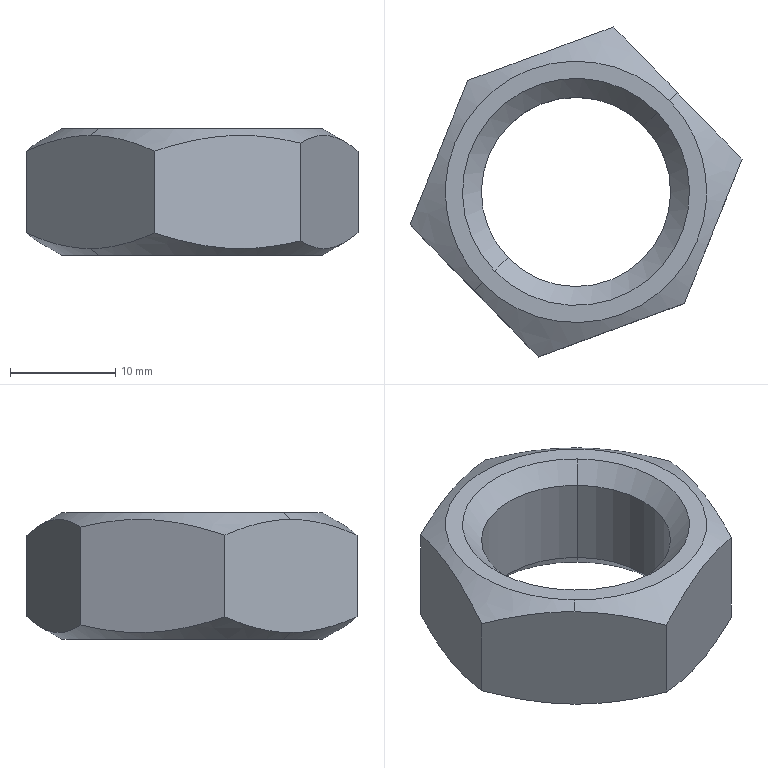Part | SolidWorks | features BaseBody 1 | 1 solid | 18 faces | box 31.577 x 31.388 x 12 mm | volume 4193 mm3 | cone 8 | plane 8 | cylinder 2 | commonest cylinder face diameters 18 x2
STEP:
#1=CARTESIAN_POINT('',(-38.01,-43.83,139.05));
#2=VERTEX_POINT('',#1);
#3=CARTESIAN_POINT('',(-50.916,-56.377,139.05));
#4=VERTEX_POINT('',#3);
#5=CARTESIAN_POINT('',(-44.463,-50.104,139.05));
#6=DIRECTION('',(0.,0.,1.));
#7=DIRECTION('',(-0.717,-0.697,0.));
#8=AXIS2_PLACEMENT_3D('',#5,#6,#7);
#9=CIRCLE('',#8,9.);
#10=EDGE_CURVE('',#2,#4,#9,.T.);
#11=ORIENTED_EDGE('',*,*,#10,.T.);
#12=CARTESIAN_POINT('',(-50.916,-56.377,130.65));
#13=VERTEX_POINT('',#12);
#14=CARTESIAN_POINT('',(-50.916,-56.377,140.85));
#15=DIRECTION('',(0.,0.,-1.));
#16=VECTOR('',#15,1000.);
#17=LINE('',#14,#16);
#18=EDGE_CURVE('',#4,#13,#17,.T.);
#19=ORIENTED_EDGE('',*,*,#18,.T.);
#20=CARTESIAN_POINT('',(-38.01,-43.83,130.65));
#21=VERTEX_POINT('',#20);
#22=CARTESIAN_POINT('',(-44.463,-50.104,130.65));
#23=DIRECTION('',(0.,0.,-1.));
#24=DIRECTION('',(-0.717,-0.697,0.));
#25=AXIS2_PLACEMENT_3D('',#22,#23,#24);
#26=CIRCLE('',#25,9.);
#27=EDGE_CURVE('',#13,#21,#26,.T.);
#28=ORIENTED_EDGE('',*,*,#27,.T.);
#29=CARTESIAN_POINT('',(-38.01,-43.83,140.85));
#30=DIRECTION('',(0.,0.,-1.));
#31=VECTOR('',#30,1000.);
#32=LINE('',#29,#31);
#33=EDGE_CURVE('',#2,#21,#32,.T.);
#34=ORIENTED_EDGE('',*,*,#33,.F.);
#35=EDGE_LOOP('',(#11,#19,#28,#34));
#36=FACE_OUTER_BOUND('',#35,.T.);
#37=CARTESIAN_POINT('',(-44.463,-50.104,140.85));
#38=DIRECTION('',(0.,0.,-1.));
#39=DIRECTION('',(0.717,0.697,0.));
#40=AXIS2_PLACEMENT_3D('',#37,#38,#39);
#41=CYLINDRICAL_SURFACE('',#40,9.);
#42=ADVANCED_FACE('',(#36),#41,.F.);
#43=ORIENTED_EDGE('',*,*,#10,.F.);
#44=CARTESIAN_POINT('',(-36.719,-42.576,140.85));
#45=VERTEX_POINT('',#44);
#46=CARTESIAN_POINT('',(-38.01,-43.83,139.05));
#47=DIRECTION('',(0.507,0.4929,0.7071));
#48=VECTOR('',#47,1000.);
#49=LINE('',#46,#48);
#50=EDGE_CURVE('',#2,#45,#49,.T.);
#51=ORIENTED_EDGE('',*,*,#50,.T.);
#52=CARTESIAN_POINT('',(-52.207,-57.632,140.85));
#53=VERTEX_POINT('',#52);
#54=CARTESIAN_POINT('',(-44.463,-50.104,140.85));
#55=DIRECTION('',(0.,0.,-1.));
#56=DIRECTION('',(-0.717,-0.697,0.));
#57=AXIS2_PLACEMENT_3D('',#54,#55,#56);
#58=CIRCLE('',#57,10.8);
#59=EDGE_CURVE('',#53,#45,#58,.T.);
#60=ORIENTED_EDGE('',*,*,#59,.F.);
#61=CARTESIAN_POINT('',(-50.916,-56.377,139.05));
#62=DIRECTION('',(-0.507,-0.4929,0.7071));
#63=VECTOR('',#62,1000.);
#64=LINE('',#61,#63);
#65=EDGE_CURVE('',#4,#53,#64,.T.);
#66=ORIENTED_EDGE('',*,*,#65,.F.);
#67=EDGE_LOOP('',(#43,#51,#60,#66));
#68=FACE_OUTER_BOUND('',#67,.T.);
#69=CARTESIAN_POINT('',(-44.463,-50.104,139.05));
#70=DIRECTION('',(0.,0.,1.));
#71=DIRECTION('',(-0.717,-0.697,0.));
#72=AXIS2_PLACEMENT_3D('',#69,#70,#71);
#73=CONICAL_SURFACE('',#72,9.,0.7854);
#74=ADVANCED_FACE('',(#68),#73,.F.);
#75=ORIENTED_EDGE('',*,*,#27,.F.);
#76=CARTESIAN_POINT('',(-52.207,-57.632,128.85));
#77=VERTEX_POINT('',#76);
#78=CARTESIAN_POINT('',(-52.207,-57.632,128.85));
#79=DIRECTION('',(-0.507,-0.4929,-0.7071));
#80=VECTOR('',#79,1000.);
#81=LINE('',#78,#80);
#82=EDGE_CURVE('',#13,#77,#81,.T.);
#83=ORIENTED_EDGE('',*,*,#82,.T.);
#84=CARTESIAN_POINT('',(-36.719,-42.576,128.85));
#85=VERTEX_POINT('',#84);
#86=CARTESIAN_POINT('',(-44.463,-50.104,128.85));
#87=DIRECTION('',(0.,0.,1.));
#88=DIRECTION('',(-0.717,-0.697,0.));
#89=AXIS2_PLACEMENT_3D('',#86,#87,#88);
#90=CIRCLE('',#89,10.8);
#91=EDGE_CURVE('',#85,#77,#90,.T.);
#92=ORIENTED_EDGE('',*,*,#91,.F.);
#93=CARTESIAN_POINT('',(-36.719,-42.576,128.85));
#94=DIRECTION('',(0.507,0.4929,-0.7071));
#95=VECTOR('',#94,1000.);
#96=LINE('',#93,#95);
#97=EDGE_CURVE('',#21,#85,#96,.T.);
#98=ORIENTED_EDGE('',*,*,#97,.F.);
#99=EDGE_LOOP('',(#75,#83,#92,#98));
#100=FACE_OUTER_BOUND('',#99,.T.);
#101=CARTESIAN_POINT('',(-44.463,-50.104,128.85));
#102=DIRECTION('',(0.,0.,-1.));
#103=DIRECTION('',(0.717,0.697,0.));
#104=AXIS2_PLACEMENT_3D('',#101,#102,#103);
#105=CONICAL_SURFACE('',#104,10.8,0.7854);
#106=ADVANCED_FACE('',(#100),#105,.F.);
#107=CARTESIAN_POINT('',(-53.372,-58.765,128.85));
#108=VERTEX_POINT('',#107);
#109=CARTESIAN_POINT('',(-35.554,-41.443,128.85));
#110=VERTEX_POINT('',#109);
#111=CARTESIAN_POINT('',(-44.463,-50.104,128.85));
#112=DIRECTION('',(0.,0.,-1.));
#113=DIRECTION('',(0.717,0.697,0.));
#114=AXIS2_PLACEMENT_3D('',#111,#112,#113);
#115=CIRCLE('',#114,12.425);
#116=EDGE_CURVE('',#108,#110,#115,.T.);
#117=ORIENTED_EDGE('',*,*,#116,.F.);
#118=CARTESIAN_POINT('',(-54.143,-59.514,129.471));
#119=VERTEX_POINT('',#118);
#120=CARTESIAN_POINT('',(-53.372,-58.765,128.85));
#121=DIRECTION('',(-0.621,-0.6037,0.5));
#122=VECTOR('',#121,1000.);
#123=LINE('',#120,#122);
#124=EDGE_CURVE('',#108,#119,#123,.T.);
#125=ORIENTED_EDGE('',*,*,#124,.T.);
#126=CARTESIAN_POINT('',(-60.251,-53.23,130.969));
#127=VERTEX_POINT('',#126);
#128=CARTESIAN_POINT('',(-54.143,-59.514,129.471));
#129=CARTESIAN_POINT('',(-55.19,-58.437,129.471));
#130=CARTESIAN_POINT('',(-56.22,-57.377,129.618));
#131=CARTESIAN_POINT('',(-58.253,-55.286,130.144));
#132=CARTESIAN_POINT('',(-59.256,-54.254,130.52));
#133=CARTESIAN_POINT('',(-60.251,-53.23,130.969));
#134=B_SPLINE_CURVE_WITH_KNOTS('',3,(#128,#129,#130,#131,#132,#133),.UNSPECIFIED.,.F.,.F.,(4,2,4),(0.008891,0.01334,0.0178),.UNSPECIFIED.);
#135=EDGE_CURVE('',#119,#127,#134,.T.);
#136=ORIENTED_EDGE('',*,*,#135,.T.);
#137=CARTESIAN_POINT('',(-54.765,-39.506,130.21));
#138=VERTEX_POINT('',#137);
#139=CARTESIAN_POINT('',(-60.251,-53.23,130.969));
#140=CARTESIAN_POINT('',(-59.363,-51.008,130.217));
#141=CARTESIAN_POINT('',(-58.462,-48.754,129.669));
#142=CARTESIAN_POINT('',(-57.303,-45.855,129.477));
#143=CARTESIAN_POINT('',(-57.069,-45.269,129.463));
#144=CARTESIAN_POINT('',(-56.603,-44.103,129.487));
#145=CARTESIAN_POINT('',(-56.371,-43.522,129.524));
#146=CARTESIAN_POINT('',(-55.678,-41.789,129.706));
#147=CARTESIAN_POINT('',(-55.22,-40.643,129.922));
#148=CARTESIAN_POINT('',(-54.765,-39.506,130.21));
#149=B_SPLINE_CURVE_WITH_KNOTS('',3,(#139,#140,#141,#142,#143,#144,#145,#146,#147,#148),.UNSPECIFIED.,.F.,.F.,(4,2,2,2,4),(0.,0.007459,0.009324,0.01119,0.01492),.UNSPECIFIED.);
#150=EDGE_CURVE('',#127,#138,#149,.T.);
#151=ORIENTED_EDGE('',*,*,#150,.T.);
#152=CARTESIAN_POINT('',(-40.892,-34.41,130.969));
#153=VERTEX_POINT('',#152);
#154=CARTESIAN_POINT('',(-54.765,-39.506,130.21));
#155=CARTESIAN_POINT('',(-53.617,-39.084,129.922));
#156=CARTESIAN_POINT('',(-52.464,-38.661,129.707));
#157=CARTESIAN_POINT('',(-50.142,-37.808,129.464));
#158=CARTESIAN_POINT('',(-48.974,-37.379,129.438));
#159=CARTESIAN_POINT('',(-47.209,-36.731,129.55));
#160=CARTESIAN_POINT('',(-46.62,-36.514,129.613));
#161=CARTESIAN_POINT('',(-45.454,-36.086,129.782));
#162=CARTESIAN_POINT('',(-44.876,-35.874,129.889));
#163=CARTESIAN_POINT('',(-43.152,-35.24,130.266));
#164=CARTESIAN_POINT('',(-42.017,-34.823,130.592));
#165=CARTESIAN_POINT('',(-40.892,-34.41,130.969));
#166=B_SPLINE_CURVE_WITH_KNOTS('',3,(#154,#155,#156,#157,#158,#159,#160,#161,#162,#163,#164,#165),.UNSPECIFIED.,.F.,.F.,(4,2,2,2,2,4),(0.,0.003728,0.007455,0.009319,0.01118,0.01491),.UNSPECIFIED.);
#167=EDGE_CURVE('',#138,#153,#166,.T.);
#168=ORIENTED_EDGE('',*,*,#167,.T.);
#169=CARTESIAN_POINT('',(-34.783,-40.694,129.471));
#170=VERTEX_POINT('',#169);
#171=CARTESIAN_POINT('',(-40.892,-34.41,130.969));
#172=CARTESIAN_POINT('',(-39.898,-35.432,130.521));
#173=CARTESIAN_POINT('',(-38.895,-36.464,130.145));
#174=CARTESIAN_POINT('',(-37.37,-38.032,129.75));
#175=CARTESIAN_POINT('',(-36.858,-38.559,129.647));
#176=CARTESIAN_POINT('',(-35.827,-39.62,129.507));
#177=CARTESIAN_POINT('',(-35.306,-40.156,129.471));
#178=CARTESIAN_POINT('',(-34.783,-40.694,129.471));
#179=B_SPLINE_CURVE_WITH_KNOTS('',3,(#171,#172,#173,#174,#175,#176,#177,#178),.UNSPECIFIED.,.F.,.F.,(4,2,2,4),(0.,0.004445,0.006668,0.008891),.UNSPECIFIED.);
#180=EDGE_CURVE('',#153,#170,#179,.T.);
#181=ORIENTED_EDGE('',*,*,#180,.T.);
#182=CARTESIAN_POINT('',(-35.554,-41.443,128.85));
#183=DIRECTION('',(0.621,0.6037,0.5));
#184=VECTOR('',#183,1000.);
#185=LINE('',#182,#184);
#186=EDGE_CURVE('',#110,#170,#185,.T.);
#187=ORIENTED_EDGE('',*,*,#186,.F.);
#188=EDGE_LOOP('',(#117,#125,#136,#151,#168,#181,#187));
#189=FACE_OUTER_BOUND('',#188,.T.);
#190=CARTESIAN_POINT('',(-44.463,-50.104,128.85));
#191=DIRECTION('',(0.,0.,1.));
#192=DIRECTION('',(0.717,0.697,0.));
#193=AXIS2_PLACEMENT_3D('',#190,#191,#192);
#194=CONICAL_SURFACE('',#193,12.425,1.047);
#195=ADVANCED_FACE('',(#189),#194,.T.);
#196=CARTESIAN_POINT('',(-35.554,-41.443,140.85));
#197=VERTEX_POINT('',#196);
#198=CARTESIAN_POINT('',(-53.372,-58.765,140.85));
#199=VERTEX_POINT('',#198);
#200=CARTESIAN_POINT('',(-44.463,-50.104,140.85));
#201=DIRECTION('',(0.,0.,1.));
#202=DIRECTION('',(-0.717,-0.697,0.));
#203=AXIS2_PLACEMENT_3D('',#200,#201,#202);
#204=CIRCLE('',#203,12.425);
#205=EDGE_CURVE('',#197,#199,#204,.T.);
#206=ORIENTED_EDGE('',*,*,#205,.F.);
#207=CARTESIAN_POINT('',(-34.783,-40.694,140.229));
#208=VERTEX_POINT('',#207);
#209=CARTESIAN_POINT('',(-35.554,-41.443,140.85));
#210=DIRECTION('',(0.621,0.6037,-0.5));
#211=VECTOR('',#210,1000.);
#212=LINE('',#209,#211);
#213=EDGE_CURVE('',#197,#208,#212,.T.);
#214=ORIENTED_EDGE('',*,*,#213,.T.);
#215=CARTESIAN_POINT('',(-40.892,-34.41,138.731));
#216=VERTEX_POINT('',#215);
#217=CARTESIAN_POINT('',(-34.783,-40.694,140.229));
#218=CARTESIAN_POINT('',(-35.83,-39.616,140.229));
#219=CARTESIAN_POINT('',(-36.86,-38.557,140.082));
#220=CARTESIAN_POINT('',(-38.893,-36.466,139.556));
#221=CARTESIAN_POINT('',(-39.897,-35.433,139.18));
#222=CARTESIAN_POINT('',(-40.892,-34.41,138.731));
#223=B_SPLINE_CURVE_WITH_KNOTS('',3,(#217,#218,#219,#220,#221,#222),.UNSPECIFIED.,.F.,.F.,(4,2,4),(0.008891,0.01334,0.0178),.UNSPECIFIED.);
#224=EDGE_CURVE('',#208,#216,#223,.T.);
#225=ORIENTED_EDGE('',*,*,#224,.T.);
#226=CARTESIAN_POINT('',(-54.765,-39.506,139.49));
#227=VERTEX_POINT('',#226);
#228=CARTESIAN_POINT('',(-40.892,-34.41,138.731));
#229=CARTESIAN_POINT('',(-43.138,-35.235,139.483));
#230=CARTESIAN_POINT('',(-45.417,-36.072,140.031));
#231=CARTESIAN_POINT('',(-48.347,-37.149,140.223));
#232=CARTESIAN_POINT('',(-48.94,-37.366,140.237));
#233=CARTESIAN_POINT('',(-50.119,-37.799,140.213));
#234=CARTESIAN_POINT('',(-50.705,-38.015,140.176));
#235=CARTESIAN_POINT('',(-52.458,-38.659,139.994));
#236=CARTESIAN_POINT('',(-53.616,-39.084,139.778));
#237=CARTESIAN_POINT('',(-54.765,-39.506,139.49));
#238=B_SPLINE_CURVE_WITH_KNOTS('',3,(#228,#229,#230,#231,#232,#233,#234,#235,#236,#237),.UNSPECIFIED.,.F.,.F.,(4,2,2,2,4),(0.,0.007459,0.009324,0.01119,0.01492),.UNSPECIFIED.);
#239=EDGE_CURVE('',#216,#227,#238,.T.);
#240=ORIENTED_EDGE('',*,*,#239,.T.);
#241=CARTESIAN_POINT('',(-60.251,-53.23,138.731));
#242=VERTEX_POINT('',#241);
#243=CARTESIAN_POINT('',(-54.765,-39.506,139.49));
#244=CARTESIAN_POINT('',(-55.219,-40.642,139.778));
#245=CARTESIAN_POINT('',(-55.675,-41.783,139.993));
#246=CARTESIAN_POINT('',(-56.593,-44.08,140.236));
#247=CARTESIAN_POINT('',(-57.055,-45.235,140.262));
#248=CARTESIAN_POINT('',(-57.753,-46.98,140.15));
#249=CARTESIAN_POINT('',(-57.986,-47.563,140.087));
#250=CARTESIAN_POINT('',(-58.447,-48.716,139.918));
#251=CARTESIAN_POINT('',(-58.676,-49.289,139.811));
#252=CARTESIAN_POINT('',(-59.358,-50.995,139.434));
#253=CARTESIAN_POINT('',(-59.806,-52.117,139.108));
#254=CARTESIAN_POINT('',(-60.251,-53.23,138.731));
#255=B_SPLINE_CURVE_WITH_KNOTS('',3,(#243,#244,#245,#246,#247,#248,#249,#250,#251,#252,#253,#254),.UNSPECIFIED.,.F.,.F.,(4,2,2,2,2,4),(0.,0.003728,0.007455,0.009319,0.01118,0.01491),.UNSPECIFIED.);
#256=EDGE_CURVE('',#227,#242,#255,.T.);
#257=ORIENTED_EDGE('',*,*,#256,.T.);
#258=CARTESIAN_POINT('',(-54.143,-59.514,140.229));
#259=VERTEX_POINT('',#258);
#260=CARTESIAN_POINT('',(-60.251,-53.23,138.731));
#261=CARTESIAN_POINT('',(-59.257,-54.253,139.179));
#262=CARTESIAN_POINT('',(-58.255,-55.284,139.555));
#263=CARTESIAN_POINT('',(-56.73,-56.853,139.95));
#264=CARTESIAN_POINT('',(-56.218,-57.379,140.053));
#265=CARTESIAN_POINT('',(-55.187,-58.44,140.193));
#266=CARTESIAN_POINT('',(-54.666,-58.976,140.229));
#267=CARTESIAN_POINT('',(-54.143,-59.514,140.229));
#268=B_SPLINE_CURVE_WITH_KNOTS('',3,(#260,#261,#262,#263,#264,#265,#266,#267),.UNSPECIFIED.,.F.,.F.,(4,2,2,4),(0.,0.004445,0.006668,0.008891),.UNSPECIFIED.);
#269=EDGE_CURVE('',#242,#259,#268,.T.);
#270=ORIENTED_EDGE('',*,*,#269,.T.);
#271=CARTESIAN_POINT('',(-53.372,-58.765,140.85));
#272=DIRECTION('',(-0.621,-0.6037,-0.5));
#273=VECTOR('',#272,1000.);
#274=LINE('',#271,#273);
#275=EDGE_CURVE('',#199,#259,#274,.T.);
#276=ORIENTED_EDGE('',*,*,#275,.F.);
#277=EDGE_LOOP('',(#206,#214,#225,#240,#257,#270,#276));
#278=FACE_OUTER_BOUND('',#277,.T.);
#279=CARTESIAN_POINT('',(-44.463,-50.104,140.85));
#280=DIRECTION('',(0.,0.,-1.));
#281=DIRECTION('',(-0.717,-0.697,0.));
#282=AXIS2_PLACEMENT_3D('',#279,#280,#281);
#283=CONICAL_SURFACE('',#282,12.425,1.047);
#284=ADVANCED_FACE('',(#278),#283,.T.);
#285=ORIENTED_EDGE('',*,*,#213,.F.);
#286=CARTESIAN_POINT('',(-44.463,-50.104,140.85));
#287=DIRECTION('',(0.,0.,1.));
#288=DIRECTION('',(-0.717,-0.697,0.));
#289=AXIS2_PLACEMENT_3D('',#286,#287,#288);
#290=CIRCLE('',#289,12.425);
#291=EDGE_CURVE('',#199,#197,#290,.T.);
#292=ORIENTED_EDGE('',*,*,#291,.F.);
#293=ORIENTED_EDGE('',*,*,#275,.T.);
#294=CARTESIAN_POINT('',(-48.034,-65.798,138.731));
#295=VERTEX_POINT('',#294);
#296=CARTESIAN_POINT('',(-54.143,-59.514,140.229));
#297=CARTESIAN_POINT('',(-53.096,-60.591,140.229));
#298=CARTESIAN_POINT('',(-52.066,-61.651,140.082));
#299=CARTESIAN_POINT('',(-50.032,-63.742,139.556));
#300=CARTESIAN_POINT('',(-49.029,-64.774,139.18));
#301=CARTESIAN_POINT('',(-48.034,-65.798,138.731));
#302=B_SPLINE_CURVE_WITH_KNOTS('',3,(#296,#297,#298,#299,#300,#301),.UNSPECIFIED.,.F.,.F.,(4,2,4),(0.008891,0.01334,0.0178),.UNSPECIFIED.);
#303=EDGE_CURVE('',#259,#295,#302,.T.);
#304=ORIENTED_EDGE('',*,*,#303,.T.);
#305=CARTESIAN_POINT('',(-34.161,-60.701,139.49));
#306=VERTEX_POINT('',#305);
#307=CARTESIAN_POINT('',(-48.034,-65.798,138.731));
#308=CARTESIAN_POINT('',(-45.788,-64.973,139.483));
#309=CARTESIAN_POINT('',(-43.509,-64.135,140.031));
#310=CARTESIAN_POINT('',(-40.579,-63.059,140.223));
#311=CARTESIAN_POINT('',(-39.986,-62.841,140.237));
#312=CARTESIAN_POINT('',(-38.807,-62.408,140.213));
#313=CARTESIAN_POINT('',(-38.22,-62.193,140.176));
#314=CARTESIAN_POINT('',(-36.468,-61.549,139.994));
#315=CARTESIAN_POINT('',(-35.31,-61.124,139.778));
#316=CARTESIAN_POINT('',(-34.161,-60.701,139.49));
#317=B_SPLINE_CURVE_WITH_KNOTS('',3,(#307,#308,#309,#310,#311,#312,#313,#314,#315,#316),.UNSPECIFIED.,.F.,.F.,(4,2,2,2,4),(0.,0.007459,0.009324,0.01119,0.01492),.UNSPECIFIED.);
#318=EDGE_CURVE('',#295,#306,#317,.T.);
#319=ORIENTED_EDGE('',*,*,#318,.T.);
#320=CARTESIAN_POINT('',(-28.674,-46.977,138.731));
#321=VERTEX_POINT('',#320);
#322=CARTESIAN_POINT('',(-34.161,-60.701,139.49));
#323=CARTESIAN_POINT('',(-33.707,-59.566,139.778));
#324=CARTESIAN_POINT('',(-33.25,-58.425,139.993));
#325=CARTESIAN_POINT('',(-32.332,-56.128,140.236));
#326=CARTESIAN_POINT('',(-31.87,-54.972,140.262));
#327=CARTESIAN_POINT('',(-31.173,-53.227,140.15));
#328=CARTESIAN_POINT('',(-30.94,-52.644,140.087));
#329=CARTESIAN_POINT('',(-30.479,-51.491,139.918));
#330=CARTESIAN_POINT('',(-30.25,-50.919,139.811));
#331=CARTESIAN_POINT('',(-29.568,-49.213,139.434));
#332=CARTESIAN_POINT('',(-29.119,-48.09,139.108));
#333=CARTESIAN_POINT('',(-28.674,-46.977,138.731));
#334=B_SPLINE_CURVE_WITH_KNOTS('',3,(#322,#323,#324,#325,#326,#327,#328,#329,#330,#331,#332,#333),.UNSPECIFIED.,.F.,.F.,(4,2,2,2,2,4),(0.,0.003728,0.007455,0.009319,0.01118,0.01491),.UNSPECIFIED.);
#335=EDGE_CURVE('',#306,#321,#334,.T.);
#336=ORIENTED_EDGE('',*,*,#335,.T.);
#337=CARTESIAN_POINT('',(-28.674,-46.977,138.731));
#338=CARTESIAN_POINT('',(-29.668,-45.955,139.179));
#339=CARTESIAN_POINT('',(-30.671,-44.923,139.555));
#340=CARTESIAN_POINT('',(-32.196,-43.355,139.95));
#341=CARTESIAN_POINT('',(-32.708,-42.829,140.053));
#342=CARTESIAN_POINT('',(-33.739,-41.768,140.193));
#343=CARTESIAN_POINT('',(-34.26,-41.231,140.229));
#344=CARTESIAN_POINT('',(-34.783,-40.694,140.229));
#345=B_SPLINE_CURVE_WITH_KNOTS('',3,(#337,#338,#339,#340,#341,#342,#343,#344),.UNSPECIFIED.,.F.,.F.,(4,2,2,4),(0.,0.004445,0.006668,0.008891),.UNSPECIFIED.);
#346=EDGE_CURVE('',#321,#208,#345,.T.);
#347=ORIENTED_EDGE('',*,*,#346,.T.);
#348=EDGE_LOOP('',(#285,#292,#293,#304,#319,#336,#347));
#349=FACE_OUTER_BOUND('',#348,.T.);
#350=CARTESIAN_POINT('',(-44.463,-50.104,140.85));
#351=DIRECTION('',(0.,0.,-1.));
#352=DIRECTION('',(-0.717,-0.697,0.));
#353=AXIS2_PLACEMENT_3D('',#350,#351,#352);
#354=CONICAL_SURFACE('',#353,12.425,1.047);
#355=ADVANCED_FACE('',(#349),#354,.T.);
#356=ORIENTED_EDGE('',*,*,#124,.F.);
#357=CARTESIAN_POINT('',(-44.463,-50.104,128.85));
#358=DIRECTION('',(0.,0.,-1.));
#359=DIRECTION('',(0.717,0.697,0.));
#360=AXIS2_PLACEMENT_3D('',#357,#358,#359);
#361=CIRCLE('',#360,12.425);
#362=EDGE_CURVE('',#110,#108,#361,.T.);
#363=ORIENTED_EDGE('',*,*,#362,.F.);
#364=ORIENTED_EDGE('',*,*,#186,.T.);
#365=CARTESIAN_POINT('',(-28.674,-46.977,130.969));
#366=VERTEX_POINT('',#365);
#367=CARTESIAN_POINT('',(-34.783,-40.694,129.471));
#368=CARTESIAN_POINT('',(-33.736,-41.771,129.471));
#369=CARTESIAN_POINT('',(-32.706,-42.83,129.618));
#370=CARTESIAN_POINT('',(-30.673,-44.922,130.144));
#371=CARTESIAN_POINT('',(-29.669,-45.954,130.52));
#372=CARTESIAN_POINT('',(-28.674,-46.977,130.969));
#373=B_SPLINE_CURVE_WITH_KNOTS('',3,(#367,#368,#369,#370,#371,#372),.UNSPECIFIED.,.F.,.F.,(4,2,4),(0.008891,0.01334,0.0178),.UNSPECIFIED.);
#374=EDGE_CURVE('',#170,#366,#373,.T.);
#375=ORIENTED_EDGE('',*,*,#374,.T.);
#376=CARTESIAN_POINT('',(-34.161,-60.701,130.21));
#377=VERTEX_POINT('',#376);
#378=CARTESIAN_POINT('',(-28.674,-46.977,130.969));
#379=CARTESIAN_POINT('',(-29.563,-49.199,130.217));
#380=CARTESIAN_POINT('',(-30.464,-51.454,129.669));
#381=CARTESIAN_POINT('',(-31.623,-54.353,129.477));
#382=CARTESIAN_POINT('',(-31.857,-54.939,129.463));
#383=CARTESIAN_POINT('',(-32.323,-56.105,129.487));
#384=CARTESIAN_POINT('',(-32.555,-56.685,129.524));
#385=CARTESIAN_POINT('',(-33.248,-58.419,129.706));
#386=CARTESIAN_POINT('',(-33.706,-59.564,129.922));
#387=CARTESIAN_POINT('',(-34.161,-60.701,130.21));
#388=B_SPLINE_CURVE_WITH_KNOTS('',3,(#378,#379,#380,#381,#382,#383,#384,#385,#386,#387),.UNSPECIFIED.,.F.,.F.,(4,2,2,2,4),(0.,0.007459,0.009324,0.01119,0.01492),.UNSPECIFIED.);
#389=EDGE_CURVE('',#366,#377,#388,.T.);
#390=ORIENTED_EDGE('',*,*,#389,.T.);
#391=CARTESIAN_POINT('',(-48.034,-65.798,130.969));
#392=VERTEX_POINT('',#391);
#393=CARTESIAN_POINT('',(-34.161,-60.701,130.21));
#394=CARTESIAN_POINT('',(-35.309,-61.123,129.922));
#395=CARTESIAN_POINT('',(-36.462,-61.547,129.707));
#396=CARTESIAN_POINT('',(-38.784,-62.4,129.464));
#397=CARTESIAN_POINT('',(-39.952,-62.829,129.438));
#398=CARTESIAN_POINT('',(-41.716,-63.477,129.55));
#399=CARTESIAN_POINT('',(-42.306,-63.693,129.613));
#400=CARTESIAN_POINT('',(-43.471,-64.121,129.782));
#401=CARTESIAN_POINT('',(-44.05,-64.334,129.889));
#402=CARTESIAN_POINT('',(-45.774,-64.967,130.266));
#403=CARTESIAN_POINT('',(-46.909,-65.384,130.592));
#404=CARTESIAN_POINT('',(-48.034,-65.798,130.969));
#405=B_SPLINE_CURVE_WITH_KNOTS('',3,(#393,#394,#395,#396,#397,#398,#399,#400,#401,#402,#403,#404),.UNSPECIFIED.,.F.,.F.,(4,2,2,2,2,4),(0.,0.003728,0.007455,0.009319,0.01118,0.01491),.UNSPECIFIED.);
#406=EDGE_CURVE('',#377,#392,#405,.T.);
#407=ORIENTED_EDGE('',*,*,#406,.T.);
#408=CARTESIAN_POINT('',(-48.034,-65.798,130.969));
#409=CARTESIAN_POINT('',(-49.028,-64.775,130.521));
#410=CARTESIAN_POINT('',(-50.031,-63.744,130.145));
#411=CARTESIAN_POINT('',(-51.556,-62.175,129.75));
#412=CARTESIAN_POINT('',(-52.067,-61.649,129.647));
#413=CARTESIAN_POINT('',(-53.099,-60.588,129.507));
#414=CARTESIAN_POINT('',(-53.62,-60.052,129.471));
#415=CARTESIAN_POINT('',(-54.143,-59.514,129.471));
#416=B_SPLINE_CURVE_WITH_KNOTS('',3,(#408,#409,#410,#411,#412,#413,#414,#415),.UNSPECIFIED.,.F.,.F.,(4,2,2,4),(0.,0.004445,0.006668,0.008891),.UNSPECIFIED.);
#417=EDGE_CURVE('',#392,#119,#416,.T.);
#418=ORIENTED_EDGE('',*,*,#417,.T.);
#419=EDGE_LOOP('',(#356,#363,#364,#375,#390,#407,#418));
#420=FACE_OUTER_BOUND('',#419,.T.);
#421=CARTESIAN_POINT('',(-44.463,-50.104,128.85));
#422=DIRECTION('',(0.,0.,1.));
#423=DIRECTION('',(0.717,0.697,0.));
#424=AXIS2_PLACEMENT_3D('',#421,#422,#423);
#425=CONICAL_SURFACE('',#424,12.425,1.047);
#426=ADVANCED_FACE('',(#420),#425,.T.);
#427=ORIENTED_EDGE('',*,*,#82,.F.);
#428=CARTESIAN_POINT('',(-44.463,-50.104,130.65));
#429=DIRECTION('',(0.,0.,-1.));
#430=DIRECTION('',(-0.717,-0.697,0.));
#431=AXIS2_PLACEMENT_3D('',#428,#429,#430);
#432=CIRCLE('',#431,9.);
#433=EDGE_CURVE('',#21,#13,#432,.T.);
#434=ORIENTED_EDGE('',*,*,#433,.F.);
#435=ORIENTED_EDGE('',*,*,#97,.T.);
#436=CARTESIAN_POINT('',(-44.463,-50.104,128.85));
#437=DIRECTION('',(0.,0.,1.));
#438=DIRECTION('',(-0.717,-0.697,0.));
#439=AXIS2_PLACEMENT_3D('',#436,#437,#438);
#440=CIRCLE('',#439,10.8);
#441=EDGE_CURVE('',#77,#85,#440,.T.);
#442=ORIENTED_EDGE('',*,*,#441,.F.);
#443=EDGE_LOOP('',(#427,#434,#435,#442));
#444=FACE_OUTER_BOUND('',#443,.T.);
#445=CARTESIAN_POINT('',(-44.463,-50.104,128.85));
#446=DIRECTION('',(0.,0.,-1.));
#447=DIRECTION('',(0.717,0.697,0.));
#448=AXIS2_PLACEMENT_3D('',#445,#446,#447);
#449=CONICAL_SURFACE('',#448,10.8,0.7854);
#450=ADVANCED_FACE('',(#444),#449,.F.);
#451=ORIENTED_EDGE('',*,*,#50,.F.);
#452=CARTESIAN_POINT('',(-44.463,-50.104,139.05));
#453=DIRECTION('',(0.,0.,1.));
#454=DIRECTION('',(-0.717,-0.697,0.));
#455=AXIS2_PLACEMENT_3D('',#452,#453,#454);
#456=CIRCLE('',#455,9.);
#457=EDGE_CURVE('',#4,#2,#456,.T.);
#458=ORIENTED_EDGE('',*,*,#457,.F.);
#459=ORIENTED_EDGE('',*,*,#65,.T.);
#460=CARTESIAN_POINT('',(-44.463,-50.104,140.85));
#461=DIRECTION('',(0.,0.,-1.));
#462=DIRECTION('',(-0.717,-0.697,0.));
#463=AXIS2_PLACEMENT_3D('',#460,#461,#462);
#464=CIRCLE('',#463,10.8);
#465=EDGE_CURVE('',#45,#53,#464,.T.);
#466=ORIENTED_EDGE('',*,*,#465,.F.);
#467=EDGE_LOOP('',(#451,#458,#459,#466));
#468=FACE_OUTER_BOUND('',#467,.T.);
#469=CARTESIAN_POINT('',(-44.463,-50.104,139.05));
#470=DIRECTION('',(0.,0.,1.));
#471=DIRECTION('',(-0.717,-0.697,0.));
#472=AXIS2_PLACEMENT_3D('',#469,#470,#471);
#473=CONICAL_SURFACE('',#472,9.,0.7854);
#474=ADVANCED_FACE('',(#468),#473,.F.);
#475=ORIENTED_EDGE('',*,*,#18,.F.);
#476=ORIENTED_EDGE('',*,*,#457,.T.);
#477=ORIENTED_EDGE('',*,*,#33,.T.);
#478=ORIENTED_EDGE('',*,*,#433,.T.);
#479=EDGE_LOOP('',(#475,#476,#477,#478));
#480=FACE_OUTER_BOUND('',#479,.T.);
#481=CARTESIAN_POINT('',(-44.463,-50.104,140.85));
#482=DIRECTION('',(0.,0.,-1.));
#483=DIRECTION('',(0.717,0.697,0.));
#484=AXIS2_PLACEMENT_3D('',#481,#482,#483);
#485=CYLINDRICAL_SURFACE('',#484,9.);
#486=ADVANCED_FACE('',(#480),#485,.F.);
#487=ORIENTED_EDGE('',*,*,#362,.T.);
#488=ORIENTED_EDGE('',*,*,#116,.T.);
#489=EDGE_LOOP('',(#487,#488));
#490=FACE_OUTER_BOUND('',#489,.T.);
#491=ORIENTED_EDGE('',*,*,#91,.T.);
#492=ORIENTED_EDGE('',*,*,#441,.T.);
#493=EDGE_LOOP('',(#491,#492));
#494=FACE_BOUND('',#493,.T.);
#495=CARTESIAN_POINT('',(-39.647,-74.426,128.85));
#496=DIRECTION('',(0.,0.,1.));
#497=DIRECTION('',(1.,0.,0.));
#498=AXIS2_PLACEMENT_3D('',#495,#496,#497);
#499=PLANE('',#498);
#500=ADVANCED_FACE('',(#490,#494),#499,.F.);
#501=ORIENTED_EDGE('',*,*,#291,.T.);
#502=ORIENTED_EDGE('',*,*,#205,.T.);
#503=EDGE_LOOP('',(#501,#502));
#504=FACE_OUTER_BOUND('',#503,.T.);
#505=ORIENTED_EDGE('',*,*,#59,.T.);
#506=ORIENTED_EDGE('',*,*,#465,.T.);
#507=EDGE_LOOP('',(#505,#506));
#508=FACE_BOUND('',#507,.T.);
#509=CARTESIAN_POINT('',(-39.647,-74.426,140.85));
#510=DIRECTION('',(0.,0.,1.));
#511=DIRECTION('',(1.,0.,0.));
#512=AXIS2_PLACEMENT_3D('',#509,#510,#511);
#513=PLANE('',#512);
#514=ADVANCED_FACE('',(#504,#508),#513,.T.);
#515=ORIENTED_EDGE('',*,*,#318,.F.);
#516=CARTESIAN_POINT('',(-48.034,-65.798,140.85));
#517=DIRECTION('',(0.,0.,-1.));
#518=VECTOR('',#517,1000.);
#519=LINE('',#516,#518);
#520=EDGE_CURVE('',#295,#392,#519,.T.);
#521=ORIENTED_EDGE('',*,*,#520,.T.);
#522=ORIENTED_EDGE('',*,*,#406,.F.);
#523=CARTESIAN_POINT('',(-34.161,-60.701,140.85));
#524=DIRECTION('',(0.,0.,-1.));
#525=VECTOR('',#524,1000.);
#526=LINE('',#523,#525);
#527=EDGE_CURVE('',#306,#377,#526,.T.);
#528=ORIENTED_EDGE('',*,*,#527,.F.);
#529=EDGE_LOOP('',(#515,#521,#522,#528));
#530=FACE_OUTER_BOUND('',#529,.T.);
#531=CARTESIAN_POINT('',(-48.034,-65.798,140.85));
#532=DIRECTION('',(-0.3448,0.9387,0.));
#533=DIRECTION('',(0.,0.,1.));
#534=AXIS2_PLACEMENT_3D('',#531,#532,#533);
#535=PLANE('',#534);
#536=ADVANCED_FACE('',(#530),#535,.F.);
#537=ORIENTED_EDGE('',*,*,#269,.F.);
#538=CARTESIAN_POINT('',(-60.251,-53.23,140.85));
#539=DIRECTION('',(0.,0.,-1.));
#540=VECTOR('',#539,1000.);
#541=LINE('',#538,#540);
#542=EDGE_CURVE('',#242,#127,#541,.T.);
#543=ORIENTED_EDGE('',*,*,#542,.T.);
#544=ORIENTED_EDGE('',*,*,#135,.F.);
#545=ORIENTED_EDGE('',*,*,#417,.F.);
#546=ORIENTED_EDGE('',*,*,#520,.F.);
#547=ORIENTED_EDGE('',*,*,#303,.F.);
#548=EDGE_LOOP('',(#537,#543,#544,#545,#546,#547));
#549=FACE_OUTER_BOUND('',#548,.T.);
#550=CARTESIAN_POINT('',(-60.251,-53.23,140.85));
#551=DIRECTION('',(0.717,0.697,0.));
#552=DIRECTION('',(0.,0.,-1.));
#553=AXIS2_PLACEMENT_3D('',#550,#551,#552);
#554=PLANE('',#553);
#555=ADVANCED_FACE('',(#549),#554,.F.);
#556=ORIENTED_EDGE('',*,*,#256,.F.);
#557=CARTESIAN_POINT('',(-54.765,-39.506,140.85));
#558=DIRECTION('',(0.,0.,-1.));
#559=VECTOR('',#558,1000.);
#560=LINE('',#557,#559);
#561=EDGE_CURVE('',#227,#138,#560,.T.);
#562=ORIENTED_EDGE('',*,*,#561,.T.);
#563=ORIENTED_EDGE('',*,*,#150,.F.);
#564=ORIENTED_EDGE('',*,*,#542,.F.);
#565=EDGE_LOOP('',(#556,#562,#563,#564));
#566=FACE_OUTER_BOUND('',#565,.T.);
#567=CARTESIAN_POINT('',(-60.251,-53.23,140.85));
#568=DIRECTION('',(0.9286,-0.3712,0.));
#569=DIRECTION('',(0.,0.,-1.));
#570=AXIS2_PLACEMENT_3D('',#567,#568,#569);
#571=PLANE('',#570);
#572=ADVANCED_FACE('',(#566),#571,.F.);
#573=ORIENTED_EDGE('',*,*,#239,.F.);
#574=CARTESIAN_POINT('',(-40.892,-34.41,140.85));
#575=DIRECTION('',(0.,0.,-1.));
#576=VECTOR('',#575,1000.);
#577=LINE('',#574,#576);
#578=EDGE_CURVE('',#216,#153,#577,.T.);
#579=ORIENTED_EDGE('',*,*,#578,.T.);
#580=ORIENTED_EDGE('',*,*,#167,.F.);
#581=ORIENTED_EDGE('',*,*,#561,.F.);
#582=EDGE_LOOP('',(#573,#579,#580,#581));
#583=FACE_OUTER_BOUND('',#582,.T.);
#584=CARTESIAN_POINT('',(-40.892,-34.41,140.85));
#585=DIRECTION('',(0.3448,-0.9387,0.));
#586=DIRECTION('',(0.,0.,-1.));
#587=AXIS2_PLACEMENT_3D('',#584,#585,#586);
#588=PLANE('',#587);
#589=ADVANCED_FACE('',(#583),#588,.F.);
#590=ORIENTED_EDGE('',*,*,#346,.F.);
#591=CARTESIAN_POINT('',(-28.674,-46.977,140.85));
#592=DIRECTION('',(0.,0.,-1.));
#593=VECTOR('',#592,1000.);
#594=LINE('',#591,#593);
#595=EDGE_CURVE('',#321,#366,#594,.T.);
#596=ORIENTED_EDGE('',*,*,#595,.T.);
#597=ORIENTED_EDGE('',*,*,#374,.F.);
#598=ORIENTED_EDGE('',*,*,#180,.F.);
#599=ORIENTED_EDGE('',*,*,#578,.F.);
#600=ORIENTED_EDGE('',*,*,#224,.F.);
#601=EDGE_LOOP('',(#590,#596,#597,#598,#599,#600));
#602=FACE_OUTER_BOUND('',#601,.T.);
#603=CARTESIAN_POINT('',(-40.892,-34.41,140.85));
#604=DIRECTION('',(-0.717,-0.697,0.));
#605=DIRECTION('',(-0.697,0.717,0.));
#606=AXIS2_PLACEMENT_3D('',#603,#604,#605);
#607=PLANE('',#606);
#608=ADVANCED_FACE('',(#602),#607,.F.);
#609=ORIENTED_EDGE('',*,*,#335,.F.);
#610=ORIENTED_EDGE('',*,*,#527,.T.);
#611=ORIENTED_EDGE('',*,*,#389,.F.);
#612=ORIENTED_EDGE('',*,*,#595,.F.);
#613=EDGE_LOOP('',(#609,#610,#611,#612));
#614=FACE_OUTER_BOUND('',#613,.T.);
#615=CARTESIAN_POINT('',(-28.674,-46.977,140.85));
#616=DIRECTION('',(-0.9286,0.3712,0.));
#617=DIRECTION('',(0.,0.,1.));
#618=AXIS2_PLACEMENT_3D('',#615,#616,#617);
#619=PLANE('',#618);
#620=ADVANCED_FACE('',(#614),#619,.F.);
#621=CLOSED_SHELL('',(#42,#74,#106,#195,#284,#355,#426,#450,#474,#486,#500,#514,#536,#555,#572,#589,#608,#620));
#622=MANIFOLD_SOLID_BREP('',#621);
#623=CARTESIAN_POINT('',(0.,0.,0.));
#624=DIRECTION('',(0.,0.,1.));
#625=DIRECTION('',(1.,0.,0.));
#626=AXIS2_PLACEMENT_3D('',#623,#624,#625);
#627=(LENGTH_UNIT()NAMED_UNIT(*)SI_UNIT(.MILLI.,.METRE.));
#628=UNCERTAINTY_MEASURE_WITH_UNIT(LENGTH_MEASURE(0.00001),#627,'','');
#629=(NAMED_UNIT(*)PLANE_ANGLE_UNIT()SI_UNIT($,.RADIAN.));
#630=(NAMED_UNIT(*)SI_UNIT($,.STERADIAN.)SOLID_ANGLE_UNIT());
#631=(GEOMETRIC_REPRESENTATION_CONTEXT(3)GLOBAL_UNCERTAINTY_ASSIGNED_CONTEXT((#628))GLOBAL_UNIT_ASSIGNED_CONTEXT((#627,#629,#630))REPRESENTATION_CONTEXT('',''));
#632=ADVANCED_BREP_SHAPE_REPRESENTATION('',(#622,#626),#631);